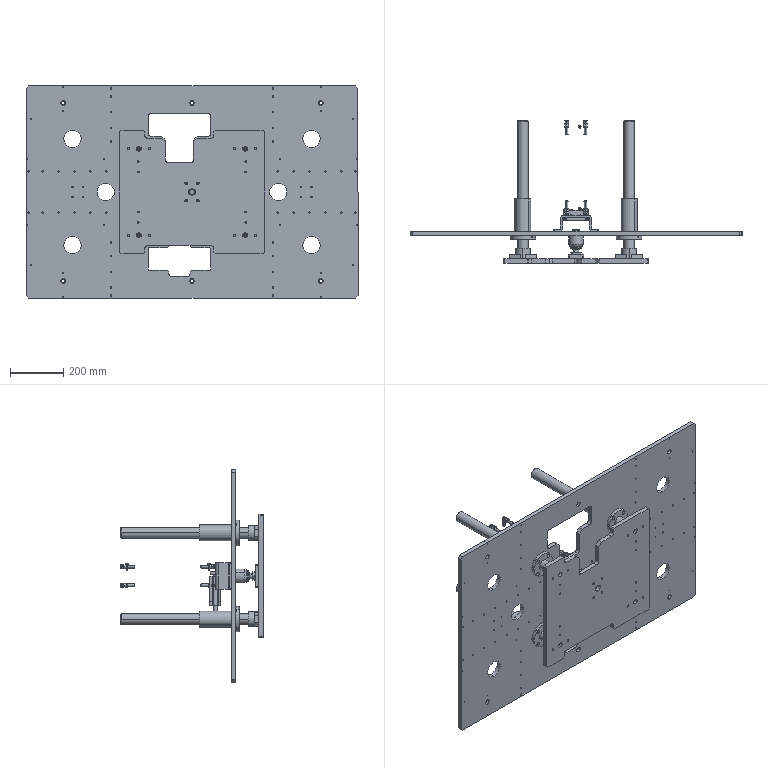Part | SolidWorks | features ReferencePattern 6, MirrorCompFeat 2, LocalLPattern 1 | 32 solids | 1603 faces | box 1250 x 536.5 x 800 mm | volume 23012589 mm3 | cylinder 728 | plane 535 | cone 302 | spline 38 | commonest cylinder face diameters 5 x136 6.8 x68 8.5 x44 9 x44 3.3 x32 10 x32